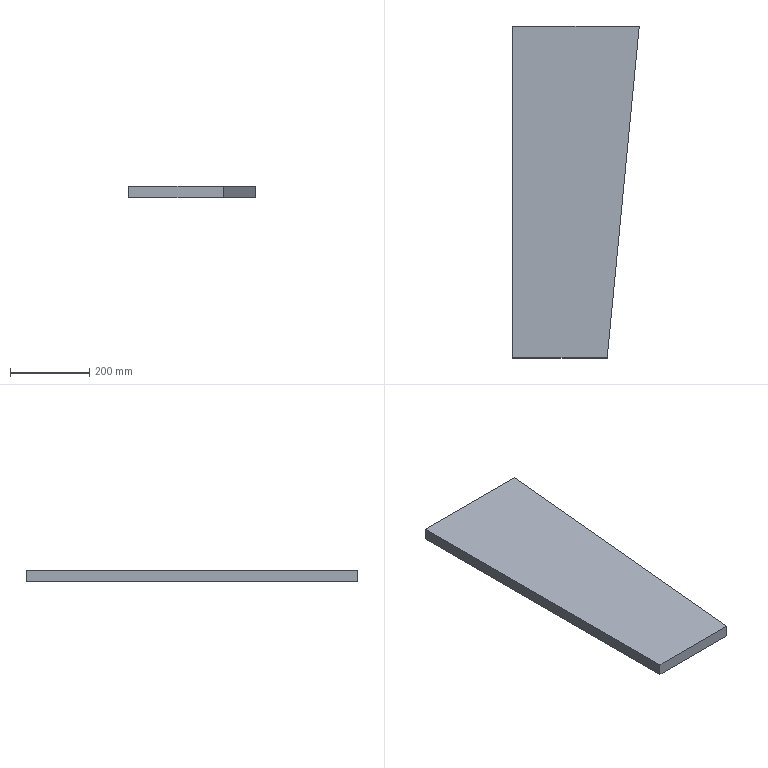Part | SolidWorks | features Extrusion 1 | 1 solid | 6 faces | box 320 x 840 x 30 mm | volume 7043400 mm3 | plane 6
STEP:
#1=CARTESIAN_POINT('',(0.,840.,0.));
#2=VERTEX_POINT('',#1);
#3=CARTESIAN_POINT('',(0.,0.,0.));
#4=VERTEX_POINT('',#3);
#5=CARTESIAN_POINT('',(0.,840.,0.));
#6=DIRECTION('',(0.,-1.,0.));
#7=VECTOR('',#6,1000.);
#8=LINE('',#5,#7);
#9=EDGE_CURVE('',#2,#4,#8,.T.);
#10=ORIENTED_EDGE('',*,*,#9,.T.);
#11=CARTESIAN_POINT('',(0.,0.,30.));
#12=VERTEX_POINT('',#11);
#13=CARTESIAN_POINT('',(0.,0.,30.));
#14=DIRECTION('',(0.,0.,-1.));
#15=VECTOR('',#14,1000.);
#16=LINE('',#13,#15);
#17=EDGE_CURVE('',#12,#4,#16,.T.);
#18=ORIENTED_EDGE('',*,*,#17,.F.);
#19=CARTESIAN_POINT('',(0.,840.,30.));
#20=VERTEX_POINT('',#19);
#21=CARTESIAN_POINT('',(0.,840.,30.));
#22=DIRECTION('',(0.,-1.,0.));
#23=VECTOR('',#22,1000.);
#24=LINE('',#21,#23);
#25=EDGE_CURVE('',#20,#12,#24,.T.);
#26=ORIENTED_EDGE('',*,*,#25,.F.);
#27=CARTESIAN_POINT('',(0.,840.,30.));
#28=DIRECTION('',(0.,0.,-1.));
#29=VECTOR('',#28,1000.);
#30=LINE('',#27,#29);
#31=EDGE_CURVE('',#20,#2,#30,.T.);
#32=ORIENTED_EDGE('',*,*,#31,.T.);
#33=EDGE_LOOP('',(#10,#18,#26,#32));
#34=FACE_OUTER_BOUND('',#33,.T.);
#35=CARTESIAN_POINT('',(0.,840.,30.));
#36=DIRECTION('',(1.,0.,0.));
#37=DIRECTION('',(0.,1.,0.));
#38=AXIS2_PLACEMENT_3D('',#35,#36,#37);
#39=PLANE('',#38);
#40=ADVANCED_FACE('',(#34),#39,.F.);
#41=CARTESIAN_POINT('',(239.,0.,0.));
#42=VERTEX_POINT('',#41);
#43=CARTESIAN_POINT('',(0.,0.,0.));
#44=DIRECTION('',(1.,0.,0.));
#45=VECTOR('',#44,1000.);
#46=LINE('',#43,#45);
#47=EDGE_CURVE('',#4,#42,#46,.T.);
#48=ORIENTED_EDGE('',*,*,#47,.T.);
#49=CARTESIAN_POINT('',(239.,0.,30.));
#50=VERTEX_POINT('',#49);
#51=CARTESIAN_POINT('',(239.,0.,30.));
#52=DIRECTION('',(0.,0.,-1.));
#53=VECTOR('',#52,1000.);
#54=LINE('',#51,#53);
#55=EDGE_CURVE('',#50,#42,#54,.T.);
#56=ORIENTED_EDGE('',*,*,#55,.F.);
#57=CARTESIAN_POINT('',(0.,0.,30.));
#58=DIRECTION('',(1.,0.,0.));
#59=VECTOR('',#58,1000.);
#60=LINE('',#57,#59);
#61=EDGE_CURVE('',#12,#50,#60,.T.);
#62=ORIENTED_EDGE('',*,*,#61,.F.);
#63=ORIENTED_EDGE('',*,*,#17,.T.);
#64=EDGE_LOOP('',(#48,#56,#62,#63));
#65=FACE_OUTER_BOUND('',#64,.T.);
#66=CARTESIAN_POINT('',(0.,0.,30.));
#67=DIRECTION('',(0.,1.,0.));
#68=DIRECTION('',(0.,0.,1.));
#69=AXIS2_PLACEMENT_3D('',#66,#67,#68);
#70=PLANE('',#69);
#71=ADVANCED_FACE('',(#65),#70,.F.);
#72=CARTESIAN_POINT('',(320.,840.,0.));
#73=VERTEX_POINT('',#72);
#74=CARTESIAN_POINT('',(239.,0.,0.));
#75=DIRECTION('',(0.09598,0.9954,0.));
#76=VECTOR('',#75,1000.);
#77=LINE('',#74,#76);
#78=EDGE_CURVE('',#42,#73,#77,.T.);
#79=ORIENTED_EDGE('',*,*,#78,.T.);
#80=CARTESIAN_POINT('',(320.,840.,30.));
#81=VERTEX_POINT('',#80);
#82=CARTESIAN_POINT('',(320.,840.,30.));
#83=DIRECTION('',(0.,0.,-1.));
#84=VECTOR('',#83,1000.);
#85=LINE('',#82,#84);
#86=EDGE_CURVE('',#81,#73,#85,.T.);
#87=ORIENTED_EDGE('',*,*,#86,.F.);
#88=CARTESIAN_POINT('',(239.,0.,30.));
#89=DIRECTION('',(0.09598,0.9954,0.));
#90=VECTOR('',#89,1000.);
#91=LINE('',#88,#90);
#92=EDGE_CURVE('',#50,#81,#91,.T.);
#93=ORIENTED_EDGE('',*,*,#92,.F.);
#94=ORIENTED_EDGE('',*,*,#55,.T.);
#95=EDGE_LOOP('',(#79,#87,#93,#94));
#96=FACE_OUTER_BOUND('',#95,.T.);
#97=CARTESIAN_POINT('',(239.,0.,30.));
#98=DIRECTION('',(-0.9954,0.09598,0.));
#99=DIRECTION('',(-0.09598,-0.9954,0.));
#100=AXIS2_PLACEMENT_3D('',#97,#98,#99);
#101=PLANE('',#100);
#102=ADVANCED_FACE('',(#96),#101,.F.);
#103=CARTESIAN_POINT('',(320.,840.,0.));
#104=DIRECTION('',(-1.,0.,0.));
#105=VECTOR('',#104,1000.);
#106=LINE('',#103,#105);
#107=EDGE_CURVE('',#73,#2,#106,.T.);
#108=ORIENTED_EDGE('',*,*,#107,.T.);
#109=ORIENTED_EDGE('',*,*,#31,.F.);
#110=CARTESIAN_POINT('',(320.,840.,30.));
#111=DIRECTION('',(-1.,0.,0.));
#112=VECTOR('',#111,1000.);
#113=LINE('',#110,#112);
#114=EDGE_CURVE('',#81,#20,#113,.T.);
#115=ORIENTED_EDGE('',*,*,#114,.F.);
#116=ORIENTED_EDGE('',*,*,#86,.T.);
#117=EDGE_LOOP('',(#108,#109,#115,#116));
#118=FACE_OUTER_BOUND('',#117,.T.);
#119=CARTESIAN_POINT('',(320.,840.,30.));
#120=DIRECTION('',(0.,-1.,0.));
#121=DIRECTION('',(0.,0.,-1.));
#122=AXIS2_PLACEMENT_3D('',#119,#120,#121);
#123=PLANE('',#122);
#124=ADVANCED_FACE('',(#118),#123,.F.);
#125=ORIENTED_EDGE('',*,*,#25,.T.);
#126=ORIENTED_EDGE('',*,*,#61,.T.);
#127=ORIENTED_EDGE('',*,*,#92,.T.);
#128=ORIENTED_EDGE('',*,*,#114,.T.);
#129=EDGE_LOOP('',(#125,#126,#127,#128));
#130=FACE_OUTER_BOUND('',#129,.T.);
#131=CARTESIAN_POINT('',(0.,0.,30.));
#132=DIRECTION('',(0.,0.,1.));
#133=DIRECTION('',(1.,0.,0.));
#134=AXIS2_PLACEMENT_3D('',#131,#132,#133);
#135=PLANE('',#134);
#136=ADVANCED_FACE('',(#130),#135,.T.);
#137=ORIENTED_EDGE('',*,*,#9,.F.);
#138=ORIENTED_EDGE('',*,*,#107,.F.);
#139=ORIENTED_EDGE('',*,*,#78,.F.);
#140=ORIENTED_EDGE('',*,*,#47,.F.);
#141=EDGE_LOOP('',(#137,#138,#139,#140));
#142=FACE_OUTER_BOUND('',#141,.T.);
#143=CARTESIAN_POINT('',(0.,0.,0.));
#144=DIRECTION('',(0.,0.,1.));
#145=DIRECTION('',(1.,0.,0.));
#146=AXIS2_PLACEMENT_3D('',#143,#144,#145);
#147=PLANE('',#146);
#148=ADVANCED_FACE('',(#142),#147,.F.);
#149=CLOSED_SHELL('',(#40,#71,#102,#124,#136,#148));
#150=MANIFOLD_SOLID_BREP('',#149);
#151=CARTESIAN_POINT('',(0.,0.,0.));
#152=DIRECTION('',(0.,0.,1.));
#153=DIRECTION('',(1.,0.,0.));
#154=AXIS2_PLACEMENT_3D('',#151,#152,#153);
#155=(LENGTH_UNIT()NAMED_UNIT(*)SI_UNIT(.MILLI.,.METRE.));
#156=UNCERTAINTY_MEASURE_WITH_UNIT(LENGTH_MEASURE(0.00001),#155,'','');
#157=(NAMED_UNIT(*)PLANE_ANGLE_UNIT()SI_UNIT($,.RADIAN.));
#158=(NAMED_UNIT(*)SI_UNIT($,.STERADIAN.)SOLID_ANGLE_UNIT());
#159=(GEOMETRIC_REPRESENTATION_CONTEXT(3)GLOBAL_UNCERTAINTY_ASSIGNED_CONTEXT((#156))GLOBAL_UNIT_ASSIGNED_CONTEXT((#155,#157,#158))REPRESENTATION_CONTEXT('',''));
#160=ADVANCED_BREP_SHAPE_REPRESENTATION('',(#150,#154),#159);